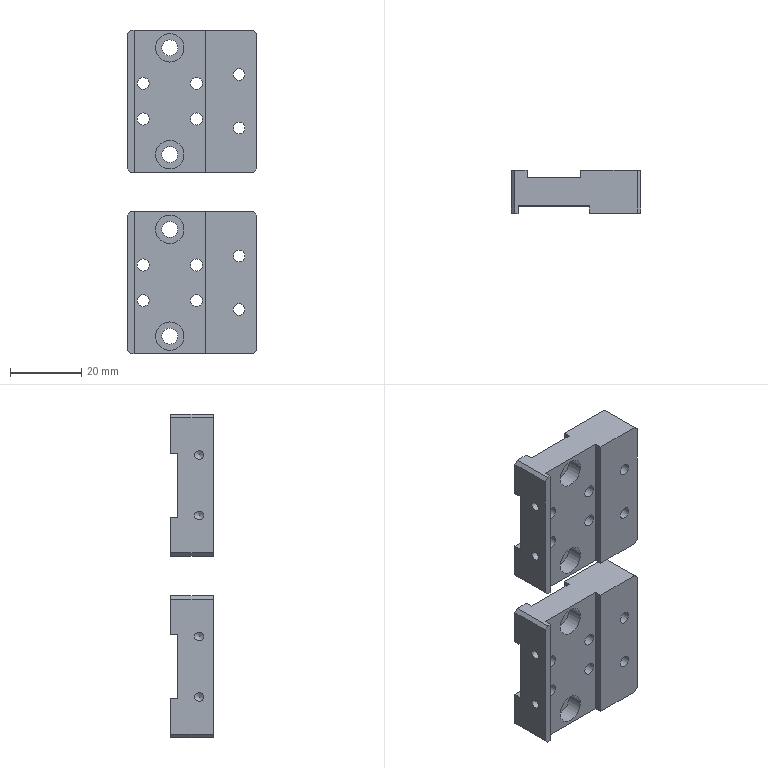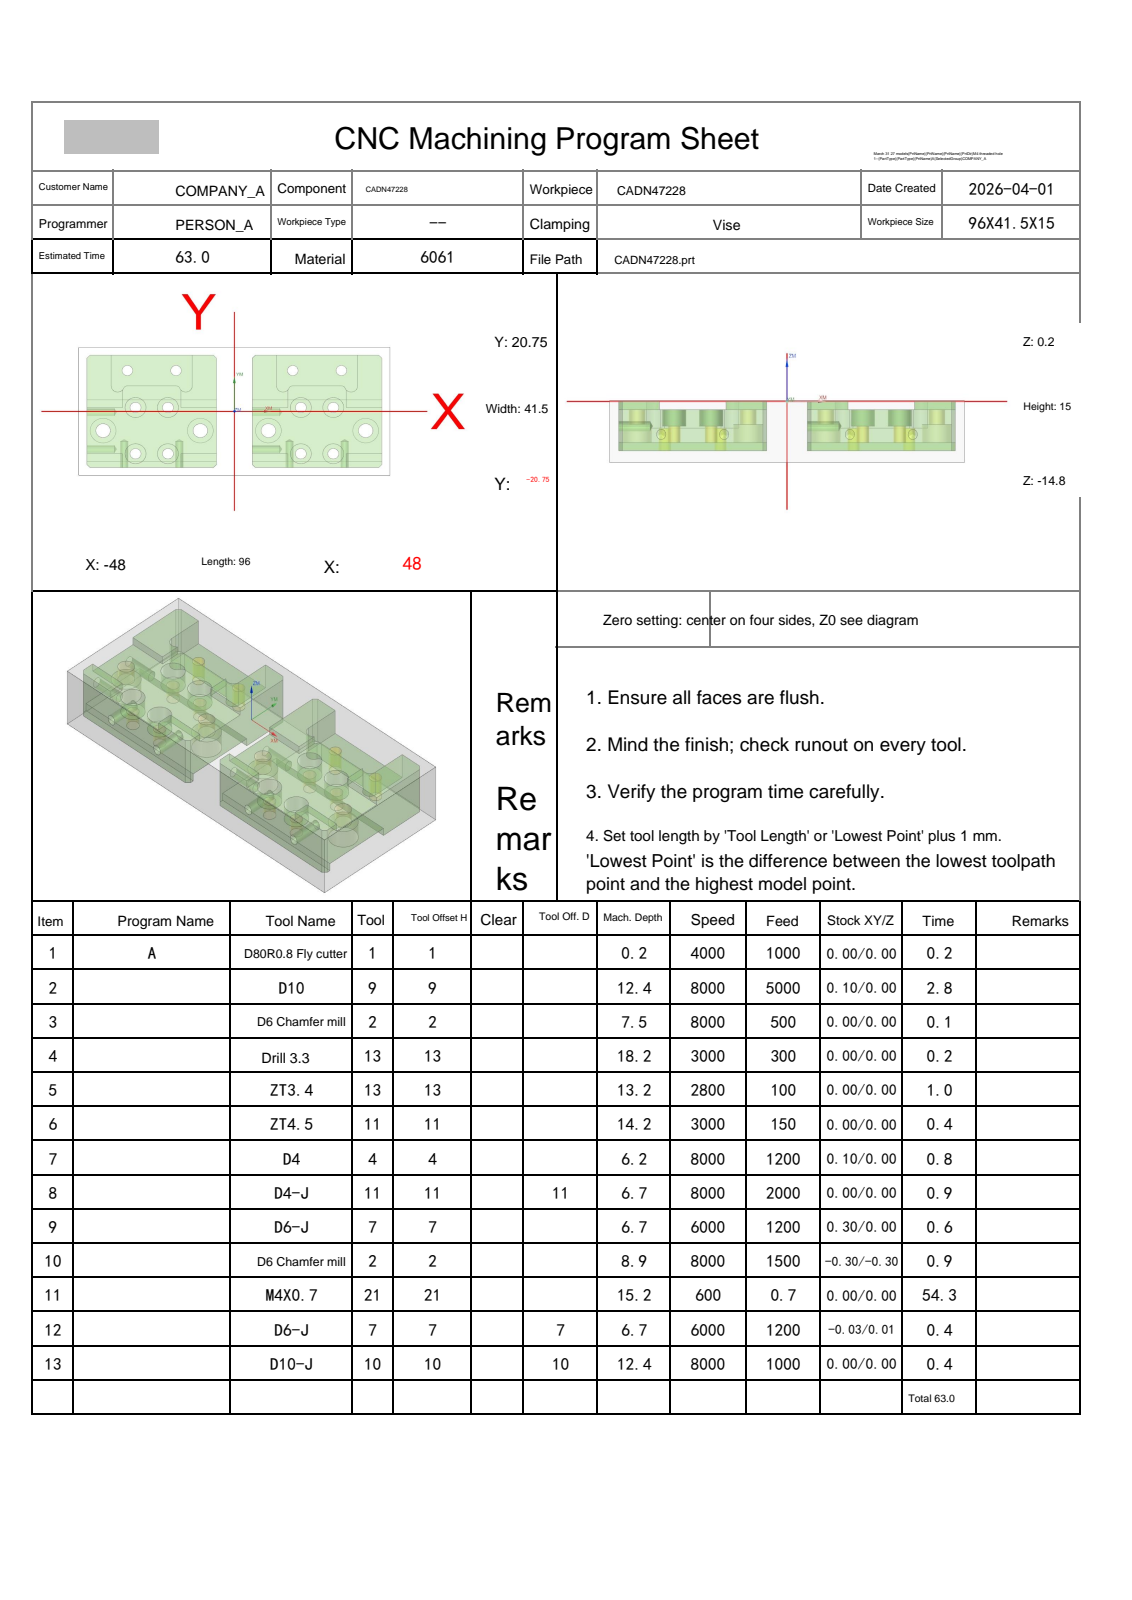NC program | NX | posted by the shop | part box 36.5 x 12 x 91 mm
Lines 1 to 1839 of 5439, first 1534 of 1837 lines:
%
O0001
(Machine time: 113.94 MIN)
(===Total Tool:9===)
(T1=D80R0.8 Fly cutter D=80.  R=0.8  D-  H01 Z=-0.   )
(T9=D10     D=10.  R=0.   D-  H09 Z=-12.2 )
(T2=D6 Chamfer mill   D=6.   R=0.   D-  H02 Z=-8.7  )
(T13=Drill 3.3  D=3.3  DR_a=118 D-  H13 Z=-17.99)
(T11=ZT4.5  D=4.5  DR_a=118 D-  H11 Z=-14.  )
(T4=D4      D=4.   R=0.   D-  H04 Z=-6.   )
(T7=D6-J    D=6.   R=0.   D-  H07 Z=-6.5  )
(T21=M4X0.7 D=3.3  DR_a=180 D-  H21 Z=-15.  )
(T10=D10-J  D=10.  R=0.   D10 H10 Z=-12.2 )
G80 G90 G17 G49 G40
G91 G28 Z0
M01
N1 T01 M06
(D80R0.8 Fly cutter  D=80. R=0.8 H=01 ce=0.00 di=0.00)
G00 G90 G54 X90.5 Y0.0 M03 S4000
G43 H01 Z20.
M08
Z2.
G01 Z0.0 F1000.
X85.5
X-85.5
X-90.5
Z2.
G00 Z20.
G91 G28 Z0.0
M05
M09
G91 G28 Z0.0
M01
N2 T09 M06
(D10  D=10. R=0. H=09 ce=0.10 di=0.00)
G00 G90 G54 X25.5 Y23.35 M03 S8000
G43 H09 Z20.
M08
Z.5
G01 X44.5 Z.449 F5000.
G02 X48.106 Y21.856 Z.438 I0.0 J-5.1
G01 X49.106 Y20.856 Z.435
G02 X50.6 Y17.25 Z.424 I-3.606 J-3.606
G01 Y-17.25 Z.332
G02 X49.106 Y-20.856 Z.321 I-5.1 J0.0
G01 X48.106 Y-21.856 Z.317
G02 X44.5 Y-23.35 Z.307 I-3.606 J3.606
G01 X6.5 Z.205
G02 X2.894 Y-21.856 Z.194 I0.0 J5.1
G01 X1.894 Y-20.856 Z.19
G02 X.4 Y-17.25 Z.18 I3.606 J3.606
G01 Y17.25 Z.088
G02 X1.894 Y20.856 Z.077 I5.1 J0.0
G01 X2.894 Y21.856 Z.073
G02 X6.5 Y23.35 Z.062 I3.606 J-3.606
G01 X44.5 Z-.039
G02 X48.106 Y21.856 Z-.05 I0.0 J-5.1
G01 X49.106 Y20.856 Z-.054
G02 X50.6 Y17.25 Z-.064 I-3.606 J-3.606
G01 Y-17.25 Z-.157
G02 X49.106 Y-20.856 Z-.167 I-5.1 J0.0
G01 X48.106 Y-21.856 Z-.171
G02 X44.5 Y-23.35 Z-.182 I-3.606 J3.606
G01 X6.5 Z-.283
G02 X2.894 Y-21.856 Z-.294 I0.0 J5.1
G01 X1.894 Y-20.856 Z-.298
G02 X.4 Y-17.25 Z-.309 I3.606 J3.606
G01 Y17.25 Z-.401
G02 X1.894 Y20.856 Z-.412 I5.1 J0.0
G01 X2.894 Y21.856 Z-.415
G02 X6.5 Y23.35 Z-.426 I3.606 J-3.606
G01 X44.5 Z-.528
G02 X48.106 Y21.856 Z-.538 I0.0 J-5.1
G01 X49.106 Y20.856 Z-.542
G02 X50.6 Y17.25 Z-.553 I-3.606 J-3.606
G01 Y-17.25 Z-.645
G02 X49.106 Y-20.856 Z-.656 I-5.1 J0.0
G01 X48.106 Y-21.856 Z-.66
G02 X44.5 Y-23.35 Z-.67 I-3.606 J3.606
G01 X6.5 Z-.772
G02 X2.894 Y-21.856 Z-.783 I0.0 J5.1
G01 X1.894 Y-20.856 Z-.786
G02 X.4 Y-17.25 Z-.797 I3.606 J3.606
G01 Y17.25 Z-.889
G02 X1.894 Y20.856 Z-.9 I5.1 J0.0
G01 X2.894 Y21.856 Z-.904
G02 X6.5 Y23.35 Z-.915 I3.606 J-3.606
G01 X44.5 Z-1.016
G02 X48.106 Y21.856 Z-1.027 I0.0 J-5.1
G01 X49.106 Y20.856 Z-1.031
G02 X50.6 Y17.25 Z-1.041 I-3.606 J-3.606
G01 Y-17.25 Z-1.134
G02 X49.106 Y-20.856 Z-1.144 I-5.1 J0.0
G01 X48.106 Y-21.856 Z-1.148
G02 X44.5 Y-23.35 Z-1.159 I-3.606 J3.606
G01 X6.5 Z-1.26
G02 X2.894 Y-21.856 Z-1.271 I0.0 J5.1
G01 X1.894 Y-20.856 Z-1.275
G02 X.4 Y-17.25 Z-1.286 I3.606 J3.606
G01 Y17.25 Z-1.378
G02 X1.894 Y20.856 Z-1.389 I5.1 J0.0
G01 X2.894 Y21.856 Z-1.392
G02 X6.5 Y23.35 Z-1.403 I3.606 J-3.606
G01 X44.5 Z-1.505
G02 X48.106 Y21.856 Z-1.515 I0.0 J-5.1
G01 X49.106 Y20.856 Z-1.519
G02 X50.6 Y17.25 Z-1.53 I-3.606 J-3.606
G01 Y-17.25 Z-1.622
G02 X49.106 Y-20.856 Z-1.633 I-5.1 J0.0
G01 X48.106 Y-21.856 Z-1.637
G02 X44.5 Y-23.35 Z-1.647 I-3.606 J3.606
G01 X6.5 Z-1.749
G02 X2.894 Y-21.856 Z-1.76 I0.0 J5.1
G01 X1.894 Y-20.856 Z-1.763
G02 X.4 Y-17.25 Z-1.774 I3.606 J3.606
G01 Y17.25 Z-1.866
G02 X1.894 Y20.856 Z-1.877 I5.1 J0.0
G01 X2.894 Y21.856 Z-1.881
G02 X6.5 Y23.35 Z-1.892 I3.606 J-3.606
G01 X44.5 Z-1.993
G02 X48.106 Y21.856 Z-2.004 I0.0 J-5.1
G01 X49.106 Y20.856 Z-2.008
G02 X50.6 Y17.25 Z-2.018 I-3.606 J-3.606
G01 Y-17.25 Z-2.111
G02 X49.106 Y-20.856 Z-2.121 I-5.1 J0.0
G01 X48.106 Y-21.856 Z-2.125
G02 X44.5 Y-23.35 Z-2.136 I-3.606 J3.606
G01 X6.5 Z-2.237
G02 X2.894 Y-21.856 Z-2.248 I0.0 J5.1
G01 X1.894 Y-20.856 Z-2.252
G02 X.4 Y-17.25 Z-2.263 I3.606 J3.606
G01 Y17.25 Z-2.355
G02 X1.894 Y20.856 Z-2.365 I5.1 J0.0
G01 X2.894 Y21.856 Z-2.369
G02 X6.5 Y23.35 Z-2.38 I3.606 J-3.606
G01 X44.5 Z-2.482
G02 X48.106 Y21.856 Z-2.492 I0.0 J-5.1
G01 X49.106 Y20.856 Z-2.496
G02 X50.6 Y17.25 Z-2.507 I-3.606 J-3.606
G01 Y-17.25 Z-2.599
G02 X49.106 Y-20.856 Z-2.61 I-5.1 J0.0
G01 X48.106 Y-21.856 Z-2.613
G02 X44.5 Y-23.35 Z-2.624 I-3.606 J3.606
G01 X6.5 Z-2.726
G02 X2.894 Y-21.856 Z-2.737 I0.0 J5.1
G01 X1.894 Y-20.856 Z-2.74
G02 X.4 Y-17.25 Z-2.751 I3.606 J3.606
G01 Y17.25 Z-2.843
G02 X1.894 Y20.856 Z-2.854 I5.1 J0.0
G01 X2.894 Y21.856 Z-2.858
G02 X6.5 Y23.35 Z-2.868 I3.606 J-3.606
G01 X44.5 Z-2.97
G02 X48.106 Y21.856 Z-2.981 I0.0 J-5.1
G01 X49.106 Y20.856 Z-2.985
G02 X50.6 Y17.25 Z-2.995 I-3.606 J-3.606
G01 Y-17.25 Z-3.087
G02 X49.106 Y-20.856 Z-3.098 I-5.1 J0.0
G01 X48.106 Y-21.856 Z-3.102
G02 X44.5 Y-23.35 Z-3.113 I-3.606 J3.606
G01 X6.5 Z-3.214
G02 X2.894 Y-21.856 Z-3.225 I0.0 J5.1
G01 X1.894 Y-20.856 Z-3.229
G02 X.4 Y-17.25 Z-3.239 I3.606 J3.606
G01 Y17.25 Z-3.332
G02 X1.894 Y20.856 Z-3.342 I5.1 J0.0
G01 X2.894 Y21.856 Z-3.346
G02 X6.5 Y23.35 Z-3.357 I3.606 J-3.606
G01 X44.5 Z-3.458
G02 X48.106 Y21.856 Z-3.469 I0.0 J-5.1
G01 X49.106 Y20.856 Z-3.473
G02 X50.6 Y17.25 Z-3.484 I-3.606 J-3.606
G01 Y-17.25 Z-3.576
G02 X49.106 Y-20.856 Z-3.587 I-5.1 J0.0
G01 X48.106 Y-21.856 Z-3.59
G02 X44.5 Y-23.35 Z-3.601 I-3.606 J3.606
G01 X6.5 Z-3.703
G02 X2.894 Y-21.856 Z-3.713 I0.0 J5.1
G01 X1.894 Y-20.856 Z-3.717
G02 X.4 Y-17.25 Z-3.728 I3.606 J3.606
G01 Y17.25 Z-3.82
G02 X1.894 Y20.856 Z-3.831 I5.1 J0.0
G01 X2.894 Y21.856 Z-3.835
G02 X6.5 Y23.35 Z-3.845 I3.606 J-3.606
G01 X44.5 Z-3.947
G02 X48.106 Y21.856 Z-3.958 I0.0 J-5.1
G01 X49.106 Y20.856 Z-3.961
G02 X50.6 Y17.25 Z-3.972 I-3.606 J-3.606
G01 Y-17.25 Z-4.064
G02 X49.106 Y-20.856 Z-4.075 I-5.1 J0.0
G01 X48.106 Y-21.856 Z-4.079
G02 X44.5 Y-23.35 Z-4.09 I-3.606 J3.606
G01 X6.5 Z-4.191
G02 X2.894 Y-21.856 Z-4.202 I0.0 J5.1
G01 X1.894 Y-20.856 Z-4.206
G02 X.4 Y-17.25 Z-4.216 I3.606 J3.606
G01 Y17.25 Z-4.309
G02 X1.894 Y20.856 Z-4.319 I5.1 J0.0
G01 X2.894 Y21.856 Z-4.323
G02 X6.5 Y23.35 Z-4.334 I3.606 J-3.606
G01 X44.5 Z-4.435
G02 X48.106 Y21.856 Z-4.446 I0.0 J-5.1
G01 X49.106 Y20.856 Z-4.45
G02 X50.6 Y17.25 Z-4.461 I-3.606 J-3.606
G01 Y-17.25 Z-4.553
G02 X49.106 Y-20.856 Z-4.564 I-5.1 J0.0
G01 X48.106 Y-21.856 Z-4.567
G02 X44.5 Y-23.35 Z-4.578 I-3.606 J3.606
G01 X6.5 Z-4.68
G02 X2.894 Y-21.856 Z-4.69 I0.0 J5.1
G01 X1.894 Y-20.856 Z-4.694
G02 X.4 Y-17.25 Z-4.705 I3.606 J3.606
G01 Y17.25 Z-4.797
G02 X1.894 Y20.856 Z-4.808 I5.1 J0.0
G01 X2.894 Y21.856 Z-4.812
G02 X6.5 Y23.35 Z-4.822 I3.606 J-3.606
G01 X44.5 Z-4.924
G02 X48.106 Y21.856 Z-4.935 I0.0 J-5.1
G01 X49.106 Y20.856 Z-4.938
G02 X50.6 Y17.25 Z-4.949 I-3.606 J-3.606
G01 Y-17.25 Z-5.041
G02 X49.106 Y-20.856 Z-5.052 I-5.1 J0.0
G01 X48.106 Y-21.856 Z-5.056
G02 X44.5 Y-23.35 Z-5.067 I-3.606 J3.606
G01 X6.5 Z-5.168
G02 X2.894 Y-21.856 Z-5.179 I0.0 J5.1
G01 X1.894 Y-20.856 Z-5.183
G02 X.4 Y-17.25 Z-5.193 I3.606 J3.606
G01 Y17.25 Z-5.286
G02 X1.894 Y20.856 Z-5.296 I5.1 J0.0
G01 X2.894 Y21.856 Z-5.3
G02 X6.5 Y23.35 Z-5.311 I3.606 J-3.606
G01 X44.5 Z-5.412
G02 X48.106 Y21.856 Z-5.423 I0.0 J-5.1
G01 X49.106 Y20.856 Z-5.427
G02 X50.6 Y17.25 Z-5.438 I-3.606 J-3.606
G01 Y-17.25 Z-5.53
G02 X49.106 Y-20.856 Z-5.54 I-5.1 J0.0
G01 X48.106 Y-21.856 Z-5.544
G02 X44.5 Y-23.35 Z-5.555 I-3.606 J3.606
G01 X6.5 Z-5.657
G02 X2.894 Y-21.856 Z-5.667 I0.0 J5.1
G01 X1.894 Y-20.856 Z-5.671
G02 X.4 Y-17.25 Z-5.682 I3.606 J3.606
G01 Y17.25 Z-5.774
G02 X1.894 Y20.856 Z-5.785 I5.1 J0.0
G01 X2.894 Y21.856 Z-5.788
G02 X6.5 Y23.35 Z-5.799 I3.606 J-3.606
G01 X44.5 Z-5.901
G02 X48.106 Y21.856 Z-5.912 I0.0 J-5.1
G01 X49.106 Y20.856 Z-5.915
G02 X50.6 Y17.25 Z-5.926 I-3.606 J-3.606
G01 Y-17.25 Z-6.018
G02 X49.106 Y-20.856 Z-6.029 I-5.1 J0.0
G01 X48.106 Y-21.856 Z-6.033
G02 X44.5 Y-23.35 Z-6.043 I-3.606 J3.606
G01 X6.5 Z-6.145
G02 X2.894 Y-21.856 Z-6.156 I0.0 J5.1
G01 X1.894 Y-20.856 Z-6.16
G02 X.4 Y-17.25 Z-6.17 I3.606 J3.606
G01 Y17.25 Z-6.262
G02 X1.894 Y20.856 Z-6.273 I5.1 J0.0
G01 X2.894 Y21.856 Z-6.277
G02 X6.5 Y23.35 Z-6.288 I3.606 J-3.606
G01 X44.5 Z-6.389
G02 X48.106 Y21.856 Z-6.4 I0.0 J-5.1
G01 X49.106 Y20.856 Z-6.404
G02 X50.6 Y17.25 Z-6.414 I-3.606 J-3.606
G01 Y-17.25 Z-6.507
G02 X49.106 Y-20.856 Z-6.517 I-5.1 J0.0
G01 X48.106 Y-21.856 Z-6.521
G02 X44.5 Y-23.35 Z-6.532 I-3.606 J3.606
G01 X6.5 Z-6.633
G02 X2.894 Y-21.856 Z-6.644 I0.0 J5.1
G01 X1.894 Y-20.856 Z-6.648
G02 X.4 Y-17.25 Z-6.659 I3.606 J3.606
G01 Y17.25 Z-6.751
G02 X1.894 Y20.856 Z-6.762 I5.1 J0.0
G01 X2.894 Y21.856 Z-6.765
G02 X6.5 Y23.35 Z-6.776 I3.606 J-3.606
G01 X44.5 Z-6.878
G02 X48.106 Y21.856 Z-6.888 I0.0 J-5.1
G01 X49.106 Y20.856 Z-6.892
G02 X50.6 Y17.25 Z-6.903 I-3.606 J-3.606
G01 Y-17.25 Z-6.995
G02 X49.106 Y-20.856 Z-7.006 I-5.1 J0.0
G01 X48.106 Y-21.856 Z-7.01
G02 X44.5 Y-23.35 Z-7.02 I-3.606 J3.606
G01 X6.5 Z-7.122
G02 X2.894 Y-21.856 Z-7.133 I0.0 J5.1
G01 X1.894 Y-20.856 Z-7.136
G02 X.4 Y-17.25 Z-7.147 I3.606 J3.606
G01 Y17.25 Z-7.239
G02 X1.894 Y20.856 Z-7.25 I5.1 J0.0
G01 X2.894 Y21.856 Z-7.254
G02 X6.5 Y23.35 Z-7.265 I3.606 J-3.606
G01 X44.5 Z-7.366
G02 X48.106 Y21.856 Z-7.377 I0.0 J-5.1
G01 X49.106 Y20.856 Z-7.381
G02 X50.6 Y17.25 Z-7.391 I-3.606 J-3.606
G01 Y-17.25 Z-7.484
G02 X49.106 Y-20.856 Z-7.494 I-5.1 J0.0
G01 X48.106 Y-21.856 Z-7.498
G02 X44.5 Y-23.35 Z-7.509 I-3.606 J3.606
G01 X6.5 Z-7.61
G02 X2.894 Y-21.856 Z-7.621 I0.0 J5.1
G01 X1.894 Y-20.856 Z-7.625
G02 X.4 Y-17.25 Z-7.636 I3.606 J3.606
G01 Y17.25 Z-7.728
G02 X1.894 Y20.856 Z-7.739 I5.1 J0.0
G01 X2.894 Y21.856 Z-7.742
G02 X6.5 Y23.35 Z-7.753 I3.606 J-3.606
G01 X44.5 Z-7.855
G02 X48.106 Y21.856 Z-7.865 I0.0 J-5.1
G01 X49.106 Y20.856 Z-7.869
G02 X50.6 Y17.25 Z-7.88 I-3.606 J-3.606
G01 Y-17.25 Z-7.972
G02 X49.106 Y-20.856 Z-7.983 I-5.1 J0.0
G01 X48.106 Y-21.856 Z-7.987
G02 X44.5 Y-23.35 Z-7.997 I-3.606 J3.606
G01 X6.5 Z-8.099
G02 X2.894 Y-21.856 Z-8.11 I0.0 J5.1
G01 X1.894 Y-20.856 Z-8.113
G02 X.4 Y-17.25 Z-8.124 I3.606 J3.606
G01 Y17.25 Z-8.216
G02 X1.894 Y20.856 Z-8.227 I5.1 J0.0
G01 X2.894 Y21.856 Z-8.231
G02 X6.5 Y23.35 Z-8.242 I3.606 J-3.606
G01 X44.5 Z-8.343
G02 X48.106 Y21.856 Z-8.354 I0.0 J-5.1
G01 X49.106 Y20.856 Z-8.358
G02 X50.6 Y17.25 Z-8.368 I-3.606 J-3.606
G01 Y-17.25 Z-8.461
G02 X49.106 Y-20.856 Z-8.471 I-5.1 J0.0
G01 X48.106 Y-21.856 Z-8.475
G02 X44.5 Y-23.35 Z-8.486 I-3.606 J3.606
G01 X6.5 Z-8.587
G02 X2.894 Y-21.856 Z-8.598 I0.0 J5.1
G01 X1.894 Y-20.856 Z-8.602
G02 X.4 Y-17.25 Z-8.613 I3.606 J3.606
G01 Y17.25 Z-8.705
G02 X1.894 Y20.856 Z-8.715 I5.1 J0.0
G01 X2.894 Y21.856 Z-8.719
G02 X6.5 Y23.35 Z-8.73 I3.606 J-3.606
G01 X44.5 Z-8.832
G02 X48.106 Y21.856 Z-8.842 I0.0 J-5.1
G01 X49.106 Y20.856 Z-8.846
G02 X50.6 Y17.25 Z-8.857 I-3.606 J-3.606
G01 Y-17.25 Z-8.949
G02 X49.106 Y-20.856 Z-8.96 I-5.1 J0.0
G01 X48.106 Y-21.856 Z-8.963
G02 X44.5 Y-23.35 Z-8.974 I-3.606 J3.606
G01 X6.5 Z-9.076
G02 X2.894 Y-21.856 Z-9.087 I0.0 J5.1
G01 X1.894 Y-20.856 Z-9.09
G02 X.4 Y-17.25 Z-9.101 I3.606 J3.606
G01 Y17.25 Z-9.193
G02 X1.894 Y20.856 Z-9.204 I5.1 J0.0
G01 X2.894 Y21.856 Z-9.208
G02 X6.5 Y23.35 Z-9.218 I3.606 J-3.606
G01 X44.5 Z-9.32
G02 X48.106 Y21.856 Z-9.331 I0.0 J-5.1
G01 X49.106 Y20.856 Z-9.335
G02 X50.6 Y17.25 Z-9.345 I-3.606 J-3.606
G01 Y-17.25 Z-9.437
G02 X49.106 Y-20.856 Z-9.448 I-5.1 J0.0
G01 X48.106 Y-21.856 Z-9.452
G02 X44.5 Y-23.35 Z-9.463 I-3.606 J3.606
G01 X6.5 Z-9.564
G02 X2.894 Y-21.856 Z-9.575 I0.0 J5.1
G01 X1.894 Y-20.856 Z-9.579
G02 X.4 Y-17.25 Z-9.589 I3.606 J3.606
G01 Y17.25 Z-9.682
G02 X1.894 Y20.856 Z-9.692 I5.1 J0.0
G01 X2.894 Y21.856 Z-9.696
G02 X6.5 Y23.35 Z-9.707 I3.606 J-3.606
G01 X44.5 Z-9.808
G02 X48.106 Y21.856 Z-9.819 I0.0 J-5.1
G01 X49.106 Y20.856 Z-9.823
G02 X50.6 Y17.25 Z-9.834 I-3.606 J-3.606
G01 Y-17.25 Z-9.926
G02 X49.106 Y-20.856 Z-9.937 I-5.1 J0.0
G01 X48.106 Y-21.856 Z-9.94
G02 X44.5 Y-23.35 Z-9.951 I-3.606 J3.606
G01 X6.5 Z-10.053
G02 X2.894 Y-21.856 Z-10.063 I0.0 J5.1
G01 X1.894 Y-20.856 Z-10.067
G02 X.4 Y-17.25 Z-10.078 I3.606 J3.606
G01 Y17.25 Z-10.17
G02 X1.894 Y20.856 Z-10.181 I5.1 J0.0
G01 X2.894 Y21.856 Z-10.185
G02 X6.5 Y23.35 Z-10.195 I3.606 J-3.606
G01 X44.5 Z-10.297
G02 X48.106 Y21.856 Z-10.308 I0.0 J-5.1
G01 X49.106 Y20.856 Z-10.311
G02 X50.6 Y17.25 Z-10.322 I-3.606 J-3.606
G01 Y-17.25 Z-10.414
G02 X49.106 Y-20.856 Z-10.425 I-5.1 J0.0
G01 X48.106 Y-21.856 Z-10.429
G02 X44.5 Y-23.35 Z-10.44 I-3.606 J3.606
G01 X6.5 Z-10.541
G02 X2.894 Y-21.856 Z-10.552 I0.0 J5.1
G01 X1.894 Y-20.856 Z-10.556
G02 X.4 Y-17.25 Z-10.566 I3.606 J3.606
G01 Y17.25 Z-10.659
G02 X1.894 Y20.856 Z-10.669 I5.1 J0.0
G01 X2.894 Y21.856 Z-10.673
G02 X6.5 Y23.35 Z-10.684 I3.606 J-3.606
G01 X44.5 Z-10.785
G02 X48.106 Y21.856 Z-10.796 I0.0 J-5.1
G01 X49.106 Y20.856 Z-10.8
G02 X50.6 Y17.25 Z-10.811 I-3.606 J-3.606
G01 Y-17.25 Z-10.903
G02 X49.106 Y-20.856 Z-10.914 I-5.1 J0.0
G01 X48.106 Y-21.856 Z-10.917
G02 X44.5 Y-23.35 Z-10.928 I-3.606 J3.606
G01 X6.5 Z-11.03
G02 X2.894 Y-21.856 Z-11.04 I0.0 J5.1
G01 X1.894 Y-20.856 Z-11.044
G02 X.4 Y-17.25 Z-11.055 I3.606 J3.606
G01 Y17.25 Z-11.147
G02 X1.894 Y20.856 Z-11.158 I5.1 J0.0
G01 X2.894 Y21.856 Z-11.162
G02 X6.5 Y23.35 Z-11.172 I3.606 J-3.606
G01 X44.5 Z-11.274
G02 X48.106 Y21.856 Z-11.285 I0.0 J-5.1
G01 X49.106 Y20.856 Z-11.288
G02 X50.6 Y17.25 Z-11.299 I-3.606 J-3.606
G01 Y-17.25 Z-11.391
G02 X49.106 Y-20.856 Z-11.402 I-5.1 J0.0
G01 X48.106 Y-21.856 Z-11.406
G02 X44.5 Y-23.35 Z-11.417 I-3.606 J3.606
G01 X6.5 Z-11.518
G02 X2.894 Y-21.856 Z-11.529 I0.0 J5.1
G01 X1.894 Y-20.856 Z-11.533
G02 X.4 Y-17.25 Z-11.543 I3.606 J3.606
G01 Y17.25 Z-11.636
G02 X1.894 Y20.856 Z-11.646 I5.1 J0.0
G01 X2.894 Y21.856 Z-11.65
G02 X6.5 Y23.35 Z-11.661 I3.606 J-3.606
G01 X44.5 Z-11.762
G02 X48.106 Y21.856 Z-11.773 I0.0 J-5.1
G01 X49.106 Y20.856 Z-11.777
G02 X50.6 Y17.25 Z-11.788 I-3.606 J-3.606
G01 Y-17.25 Z-11.88
G02 X49.106 Y-20.856 Z-11.89 I-5.1 J0.0
G01 X48.106 Y-21.856 Z-11.894
G02 X44.5 Y-23.35 Z-11.905 I-3.606 J3.606
G01 X6.5 Z-12.007
G02 X2.894 Y-21.856 Z-12.017 I0.0 J5.1
G01 X1.894 Y-20.856 Z-12.021
G02 X.4 Y-17.25 Z-12.032 I3.606 J3.606
G01 Y17.25 Z-12.124
G02 X1.894 Y20.856 Z-12.135 I5.1 J0.0
G01 X2.894 Y21.856 Z-12.138
G02 X6.5 Y23.35 Z-12.149 I3.606 J-3.606
G01 X25.5 Z-12.2
X44.5
G02 X48.106 Y21.856 I0.0 J-5.1
G01 X49.106 Y20.856
G02 X50.6 Y17.25 I-3.606 J-3.606
G01 Y-17.25
G02 X49.106 Y-20.856 I-5.1 J0.0
G01 X48.106 Y-21.856
G02 X44.5 Y-23.35 I-3.606 J3.606
G01 X6.5
G02 X2.894 Y-21.856 I0.0 J5.1
G01 X1.894 Y-20.856
G02 X.4 Y-17.25 I3.606 J3.606
G01 Y17.25
G02 X1.894 Y20.856 I5.1 J0.0
G01 X2.894 Y21.856
G02 X6.5 Y23.35 I3.606 J-3.606
G01 X25.5
X26.
Z-11.2
G00 Z20.
X-25.5
Z.5
G01 X-6.5 Z.449
G02 X-2.894 Y21.856 Z.438 I0.0 J-5.1
G01 X-1.894 Y20.856 Z.435
G02 X-.409 Y17.547 Z.425 I-3.606 J-3.606
X-.4 Y17.25 Z.424 I-5.091 J-.297
G01 Y-17.25 Z.332
G02 X-1.894 Y-20.856 Z.321 I-5.1 J0.0
G01 X-2.894 Y-21.856 Z.317
G02 X-6.5 Y-23.35 Z.307 I-3.606 J3.606
G01 X-44.5 Z.205
G02 X-48.106 Y-21.856 Z.194 I0.0 J5.1
G01 X-49.106 Y-20.856 Z.19
G02 X-50.6 Y-17.25 Z.18 I3.606 J3.606
G01 Y17.25 Z.088
G02 X-49.106 Y20.856 Z.077 I5.1 J0.0
G01 X-48.106 Y21.856 Z.073
G02 X-44.5 Y23.35 Z.062 I3.606 J-3.606
G01 X-6.5 Z-.039
G02 X-2.894 Y21.856 Z-.05 I0.0 J-5.1
G01 X-1.894 Y20.856 Z-.054
G02 X-.409 Y17.547 Z-.064 I-3.606 J-3.606
X-.4 Y17.25 Z-.064 I-5.091 J-.297
G01 Y-17.25 Z-.157
G02 X-1.894 Y-20.856 Z-.167 I-5.1 J0.0
G01 X-2.894 Y-21.856 Z-.171
G02 X-6.5 Y-23.35 Z-.182 I-3.606 J3.606
G01 X-44.5 Z-.283
G02 X-48.106 Y-21.856 Z-.294 I0.0 J5.1
G01 X-49.106 Y-20.856 Z-.298
G02 X-50.6 Y-17.25 Z-.309 I3.606 J3.606
G01 Y17.25 Z-.401
G02 X-49.106 Y20.856 Z-.412 I5.1 J0.0
G01 X-48.106 Y21.856 Z-.415
G02 X-44.5 Y23.35 Z-.426 I3.606 J-3.606
G01 X-6.5 Z-.528
G02 X-2.894 Y21.856 Z-.538 I0.0 J-5.1
G01 X-1.894 Y20.856 Z-.542
G02 X-.409 Y17.547 Z-.552 I-3.606 J-3.606
X-.4 Y17.25 Z-.553 I-5.091 J-.297
G01 Y-17.25 Z-.645
G02 X-1.894 Y-20.856 Z-.656 I-5.1 J0.0
G01 X-2.894 Y-21.856 Z-.66
G02 X-6.5 Y-23.35 Z-.67 I-3.606 J3.606
G01 X-44.5 Z-.772
G02 X-48.106 Y-21.856 Z-.783 I0.0 J5.1
G01 X-49.106 Y-20.856 Z-.786
G02 X-50.6 Y-17.25 Z-.797 I3.606 J3.606
G01 Y17.25 Z-.889
G02 X-49.106 Y20.856 Z-.9 I5.1 J0.0
G01 X-48.106 Y21.856 Z-.904
G02 X-44.5 Y23.35 Z-.915 I3.606 J-3.606
G01 X-6.5 Z-1.016
G02 X-2.894 Y21.856 Z-1.027 I0.0 J-5.1
G01 X-1.894 Y20.856 Z-1.031
G02 X-.409 Y17.547 Z-1.041 I-3.606 J-3.606
X-.4 Y17.25 Z-1.041 I-5.091 J-.297
G01 Y-17.25 Z-1.134
G02 X-1.894 Y-20.856 Z-1.144 I-5.1 J0.0
G01 X-2.894 Y-21.856 Z-1.148
G02 X-6.5 Y-23.35 Z-1.159 I-3.606 J3.606
G01 X-44.5 Z-1.26
G02 X-48.106 Y-21.856 Z-1.271 I0.0 J5.1
G01 X-49.106 Y-20.856 Z-1.275
G02 X-50.6 Y-17.25 Z-1.286 I3.606 J3.606
G01 Y17.25 Z-1.378
G02 X-49.106 Y20.856 Z-1.389 I5.1 J0.0
G01 X-48.106 Y21.856 Z-1.392
G02 X-44.5 Y23.35 Z-1.403 I3.606 J-3.606
G01 X-6.5 Z-1.505
G02 X-2.894 Y21.856 Z-1.515 I0.0 J-5.1
G01 X-1.894 Y20.856 Z-1.519
G02 X-.409 Y17.547 Z-1.529 I-3.606 J-3.606
X-.4 Y17.25 Z-1.53 I-5.091 J-.297
G01 Y-17.25 Z-1.622
G02 X-1.894 Y-20.856 Z-1.633 I-5.1 J0.0
G01 X-2.894 Y-21.856 Z-1.637
G02 X-6.5 Y-23.35 Z-1.647 I-3.606 J3.606
G01 X-44.5 Z-1.749
G02 X-48.106 Y-21.856 Z-1.76 I0.0 J5.1
G01 X-49.106 Y-20.856 Z-1.763
G02 X-50.6 Y-17.25 Z-1.774 I3.606 J3.606
G01 Y17.25 Z-1.866
G02 X-49.106 Y20.856 Z-1.877 I5.1 J0.0
G01 X-48.106 Y21.856 Z-1.881
G02 X-44.5 Y23.35 Z-1.892 I3.606 J-3.606
G01 X-6.5 Z-1.993
G02 X-2.894 Y21.856 Z-2.004 I0.0 J-5.1
G01 X-1.894 Y20.856 Z-2.008
G02 X-.409 Y17.547 Z-2.018 I-3.606 J-3.606
X-.4 Y17.25 Z-2.018 I-5.091 J-.297
G01 Y-17.25 Z-2.111
G02 X-1.894 Y-20.856 Z-2.121 I-5.1 J0.0
G01 X-2.894 Y-21.856 Z-2.125
G02 X-6.5 Y-23.35 Z-2.136 I-3.606 J3.606
G01 X-44.5 Z-2.237
G02 X-48.106 Y-21.856 Z-2.248 I0.0 J5.1
G01 X-49.106 Y-20.856 Z-2.252
G02 X-50.6 Y-17.25 Z-2.263 I3.606 J3.606
G01 Y17.25 Z-2.355
G02 X-49.106 Y20.856 Z-2.365 I5.1 J0.0
G01 X-48.106 Y21.856 Z-2.369
G02 X-44.5 Y23.35 Z-2.38 I3.606 J-3.606
G01 X-6.5 Z-2.482
G02 X-2.894 Y21.856 Z-2.492 I0.0 J-5.1
G01 X-1.894 Y20.856 Z-2.496
G02 X-.409 Y17.547 Z-2.506 I-3.606 J-3.606
X-.4 Y17.25 Z-2.507 I-5.091 J-.297
G01 Y-17.25 Z-2.599
G02 X-1.894 Y-20.856 Z-2.61 I-5.1 J0.0
G01 X-2.894 Y-21.856 Z-2.613
G02 X-6.5 Y-23.35 Z-2.624 I-3.606 J3.606
G01 X-44.5 Z-2.726
G02 X-48.106 Y-21.856 Z-2.737 I0.0 J5.1
G01 X-49.106 Y-20.856 Z-2.74
G02 X-50.6 Y-17.25 Z-2.751 I3.606 J3.606
G01 Y17.25 Z-2.843
G02 X-49.106 Y20.856 Z-2.854 I5.1 J0.0
G01 X-48.106 Y21.856 Z-2.858
G02 X-44.5 Y23.35 Z-2.868 I3.606 J-3.606
G01 X-6.5 Z-2.97
G02 X-2.894 Y21.856 Z-2.981 I0.0 J-5.1
G01 X-1.894 Y20.856 Z-2.985
G02 X-.409 Y17.547 Z-2.994 I-3.606 J-3.606
X-.4 Y17.25 Z-2.995 I-5.091 J-.297
G01 Y-17.25 Z-3.087
G02 X-1.894 Y-20.856 Z-3.098 I-5.1 J0.0
G01 X-2.894 Y-21.856 Z-3.102
G02 X-6.5 Y-23.35 Z-3.113 I-3.606 J3.606
G01 X-44.5 Z-3.214
G02 X-48.106 Y-21.856 Z-3.225 I0.0 J5.1
G01 X-49.106 Y-20.856 Z-3.229
G02 X-50.6 Y-17.25 Z-3.239 I3.606 J3.606
G01 Y17.25 Z-3.332
G02 X-49.106 Y20.856 Z-3.342 I5.1 J0.0
G01 X-48.106 Y21.856 Z-3.346
G02 X-44.5 Y23.35 Z-3.357 I3.606 J-3.606
G01 X-6.5 Z-3.458
G02 X-2.894 Y21.856 Z-3.469 I0.0 J-5.1
G01 X-1.894 Y20.856 Z-3.473
G02 X-.409 Y17.547 Z-3.483 I-3.606 J-3.606
X-.4 Y17.25 Z-3.484 I-5.091 J-.297
G01 Y-17.25 Z-3.576
G02 X-1.894 Y-20.856 Z-3.587 I-5.1 J0.0
G01 X-2.894 Y-21.856 Z-3.59
G02 X-6.5 Y-23.35 Z-3.601 I-3.606 J3.606
G01 X-44.5 Z-3.703
G02 X-48.106 Y-21.856 Z-3.713 I0.0 J5.1
G01 X-49.106 Y-20.856 Z-3.717
G02 X-50.6 Y-17.25 Z-3.728 I3.606 J3.606
G01 Y17.25 Z-3.82
G02 X-49.106 Y20.856 Z-3.831 I5.1 J0.0
G01 X-48.106 Y21.856 Z-3.835
G02 X-44.5 Y23.35 Z-3.845 I3.606 J-3.606
G01 X-6.5 Z-3.947
G02 X-2.894 Y21.856 Z-3.958 I0.0 J-5.1
G01 X-1.894 Y20.856 Z-3.961
G02 X-.409 Y17.547 Z-3.971 I-3.606 J-3.606
X-.4 Y17.25 Z-3.972 I-5.091 J-.297
G01 Y-17.25 Z-4.064
G02 X-1.894 Y-20.856 Z-4.075 I-5.1 J0.0
G01 X-2.894 Y-21.856 Z-4.079
G02 X-6.5 Y-23.35 Z-4.09 I-3.606 J3.606
G01 X-44.5 Z-4.191
G02 X-48.106 Y-21.856 Z-4.202 I0.0 J5.1
G01 X-49.106 Y-20.856 Z-4.206
G02 X-50.6 Y-17.25 Z-4.216 I3.606 J3.606
G01 Y17.25 Z-4.309
G02 X-49.106 Y20.856 Z-4.319 I5.1 J0.0
G01 X-48.106 Y21.856 Z-4.323
G02 X-44.5 Y23.35 Z-4.334 I3.606 J-3.606
G01 X-6.5 Z-4.435
G02 X-2.894 Y21.856 Z-4.446 I0.0 J-5.1
G01 X-1.894 Y20.856 Z-4.45
G02 X-.409 Y17.547 Z-4.46 I-3.606 J-3.606
X-.4 Y17.25 Z-4.461 I-5.091 J-.297
G01 Y-17.25 Z-4.553
G02 X-1.894 Y-20.856 Z-4.564 I-5.1 J0.0
G01 X-2.894 Y-21.856 Z-4.567
G02 X-6.5 Y-23.35 Z-4.578 I-3.606 J3.606
G01 X-44.5 Z-4.68
G02 X-48.106 Y-21.856 Z-4.69 I0.0 J5.1
G01 X-49.106 Y-20.856 Z-4.694
G02 X-50.6 Y-17.25 Z-4.705 I3.606 J3.606
G01 Y17.25 Z-4.797
G02 X-49.106 Y20.856 Z-4.808 I5.1 J0.0
G01 X-48.106 Y21.856 Z-4.812
G02 X-44.5 Y23.35 Z-4.822 I3.606 J-3.606
G01 X-6.5 Z-4.924
G02 X-2.894 Y21.856 Z-4.935 I0.0 J-5.1
G01 X-1.894 Y20.856 Z-4.938
G02 X-.409 Y17.547 Z-4.948 I-3.606 J-3.606
X-.4 Y17.25 Z-4.949 I-5.091 J-.297
G01 Y-17.25 Z-5.041
G02 X-1.894 Y-20.856 Z-5.052 I-5.1 J0.0
G01 X-2.894 Y-21.856 Z-5.056
G02 X-6.5 Y-23.35 Z-5.067 I-3.606 J3.606
G01 X-44.5 Z-5.168
G02 X-48.106 Y-21.856 Z-5.179 I0.0 J5.1
G01 X-49.106 Y-20.856 Z-5.183
G02 X-50.6 Y-17.25 Z-5.193 I3.606 J3.606
G01 Y17.25 Z-5.286
G02 X-49.106 Y20.856 Z-5.296 I5.1 J0.0
G01 X-48.106 Y21.856 Z-5.3
G02 X-44.5 Y23.35 Z-5.311 I3.606 J-3.606
G01 X-6.5 Z-5.412
G02 X-2.894 Y21.856 Z-5.423 I0.0 J-5.1
G01 X-1.894 Y20.856 Z-5.427
G02 X-.409 Y17.547 Z-5.437 I-3.606 J-3.606
X-.4 Y17.25 Z-5.438 I-5.091 J-.297
G01 Y-17.25 Z-5.53
G02 X-1.894 Y-20.856 Z-5.54 I-5.1 J0.0
G01 X-2.894 Y-21.856 Z-5.544
G02 X-6.5 Y-23.35 Z-5.555 I-3.606 J3.606
G01 X-44.5 Z-5.657
G02 X-48.106 Y-21.856 Z-5.667 I0.0 J5.1
G01 X-49.106 Y-20.856 Z-5.671
G02 X-50.6 Y-17.25 Z-5.682 I3.606 J3.606
G01 Y17.25 Z-5.774
G02 X-49.106 Y20.856 Z-5.785 I5.1 J0.0
G01 X-48.106 Y21.856 Z-5.788
G02 X-44.5 Y23.35 Z-5.799 I3.606 J-3.606
G01 X-6.5 Z-5.901
G02 X-2.894 Y21.856 Z-5.912 I0.0 J-5.1
G01 X-1.894 Y20.856 Z-5.915
G02 X-.409 Y17.547 Z-5.925 I-3.606 J-3.606
X-.4 Y17.25 Z-5.926 I-5.091 J-.297
G01 Y-17.25 Z-6.018
G02 X-1.894 Y-20.856 Z-6.029 I-5.1 J0.0
G01 X-2.894 Y-21.856 Z-6.033
G02 X-6.5 Y-23.35 Z-6.043 I-3.606 J3.606
G01 X-44.5 Z-6.145
G02 X-48.106 Y-21.856 Z-6.156 I0.0 J5.1
G01 X-49.106 Y-20.856 Z-6.16
G02 X-50.6 Y-17.25 Z-6.17 I3.606 J3.606
G01 Y17.25 Z-6.262
G02 X-49.106 Y20.856 Z-6.273 I5.1 J0.0
G01 X-48.106 Y21.856 Z-6.277
G02 X-44.5 Y23.35 Z-6.288 I3.606 J-3.606
G01 X-6.5 Z-6.389
G02 X-2.894 Y21.856 Z-6.4 I0.0 J-5.1
G01 X-1.894 Y20.856 Z-6.404
G02 X-.409 Y17.547 Z-6.414 I-3.606 J-3.606
X-.4 Y17.25 Z-6.414 I-5.091 J-.297
G01 Y-17.25 Z-6.507
G02 X-1.894 Y-20.856 Z-6.517 I-5.1 J0.0
G01 X-2.894 Y-21.856 Z-6.521
G02 X-6.5 Y-23.35 Z-6.532 I-3.606 J3.606
G01 X-44.5 Z-6.633
G02 X-48.106 Y-21.856 Z-6.644 I0.0 J5.1
G01 X-49.106 Y-20.856 Z-6.648
G02 X-50.6 Y-17.25 Z-6.659 I3.606 J3.606
G01 Y17.25 Z-6.751
G02 X-49.106 Y20.856 Z-6.762 I5.1 J0.0
G01 X-48.106 Y21.856 Z-6.765
G02 X-44.5 Y23.35 Z-6.776 I3.606 J-3.606
G01 X-6.5 Z-6.878
G02 X-2.894 Y21.856 Z-6.888 I0.0 J-5.1
G01 X-1.894 Y20.856 Z-6.892
G02 X-.409 Y17.547 Z-6.902 I-3.606 J-3.606
X-.4 Y17.25 Z-6.903 I-5.091 J-.297
G01 Y-17.25 Z-6.995
G02 X-1.894 Y-20.856 Z-7.006 I-5.1 J0.0
G01 X-2.894 Y-21.856 Z-7.01
G02 X-6.5 Y-23.35 Z-7.02 I-3.606 J3.606
G01 X-44.5 Z-7.122
G02 X-48.106 Y-21.856 Z-7.133 I0.0 J5.1
G01 X-49.106 Y-20.856 Z-7.136
G02 X-50.6 Y-17.25 Z-7.147 I3.606 J3.606
G01 Y17.25 Z-7.239
G02 X-49.106 Y20.856 Z-7.25 I5.1 J0.0
G01 X-48.106 Y21.856 Z-7.254
G02 X-44.5 Y23.35 Z-7.265 I3.606 J-3.606
G01 X-6.5 Z-7.366
G02 X-2.894 Y21.856 Z-7.377 I0.0 J-5.1
G01 X-1.894 Y20.856 Z-7.381
G02 X-.409 Y17.547 Z-7.391 I-3.606 J-3.606
X-.4 Y17.25 Z-7.391 I-5.091 J-.297
G01 Y-17.25 Z-7.484
G02 X-1.894 Y-20.856 Z-7.494 I-5.1 J0.0
G01 X-2.894 Y-21.856 Z-7.498
G02 X-6.5 Y-23.35 Z-7.509 I-3.606 J3.606
G01 X-44.5 Z-7.61
G02 X-48.106 Y-21.856 Z-7.621 I0.0 J5.1
G01 X-49.106 Y-20.856 Z-7.625
G02 X-50.6 Y-17.25 Z-7.636 I3.606 J3.606
G01 Y17.25 Z-7.728
G02 X-49.106 Y20.856 Z-7.739 I5.1 J0.0
G01 X-48.106 Y21.856 Z-7.742
G02 X-44.5 Y23.35 Z-7.753 I3.606 J-3.606
G01 X-6.5 Z-7.855
G02 X-2.894 Y21.856 Z-7.865 I0.0 J-5.1
G01 X-1.894 Y20.856 Z-7.869
G02 X-.409 Y17.547 Z-7.879 I-3.606 J-3.606
X-.4 Y17.25 Z-7.88 I-5.091 J-.297
G01 Y-17.25 Z-7.972
G02 X-1.894 Y-20.856 Z-7.983 I-5.1 J0.0
G01 X-2.894 Y-21.856 Z-7.987
G02 X-6.5 Y-23.35 Z-7.997 I-3.606 J3.606
G01 X-44.5 Z-8.099
G02 X-48.106 Y-21.856 Z-8.11 I0.0 J5.1
G01 X-49.106 Y-20.856 Z-8.113
G02 X-50.6 Y-17.25 Z-8.124 I3.606 J3.606
G01 Y17.25 Z-8.216
G02 X-49.106 Y20.856 Z-8.227 I5.1 J0.0
G01 X-48.106 Y21.856 Z-8.231
G02 X-44.5 Y23.35 Z-8.242 I3.606 J-3.606
G01 X-6.5 Z-8.343
G02 X-2.894 Y21.856 Z-8.354 I0.0 J-5.1
G01 X-1.894 Y20.856 Z-8.358
G02 X-.409 Y17.547 Z-8.368 I-3.606 J-3.606
X-.4 Y17.25 Z-8.368 I-5.091 J-.297
G01 Y-17.25 Z-8.461
G02 X-1.894 Y-20.856 Z-8.471 I-5.1 J0.0
G01 X-2.894 Y-21.856 Z-8.475
G02 X-6.5 Y-23.35 Z-8.486 I-3.606 J3.606
G01 X-44.5 Z-8.587
G02 X-48.106 Y-21.856 Z-8.598 I0.0 J5.1
G01 X-49.106 Y-20.856 Z-8.602
G02 X-50.6 Y-17.25 Z-8.613 I3.606 J3.606
G01 Y17.25 Z-8.705
G02 X-49.106 Y20.856 Z-8.715 I5.1 J0.0
G01 X-48.106 Y21.856 Z-8.719
G02 X-44.5 Y23.35 Z-8.73 I3.606 J-3.606
G01 X-6.5 Z-8.832
G02 X-2.894 Y21.856 Z-8.842 I0.0 J-5.1
G01 X-1.894 Y20.856 Z-8.846
G02 X-.409 Y17.547 Z-8.856 I-3.606 J-3.606
X-.4 Y17.25 Z-8.857 I-5.091 J-.297
G01 Y-17.25 Z-8.949
G02 X-1.894 Y-20.856 Z-8.96 I-5.1 J0.0
G01 X-2.894 Y-21.856 Z-8.963
G02 X-6.5 Y-23.35 Z-8.974 I-3.606 J3.606
G01 X-44.5 Z-9.076
G02 X-48.106 Y-21.856 Z-9.087 I0.0 J5.1
G01 X-49.106 Y-20.856 Z-9.09
G02 X-50.6 Y-17.25 Z-9.101 I3.606 J3.606
G01 Y17.25 Z-9.193
G02 X-49.106 Y20.856 Z-9.204 I5.1 J0.0
G01 X-48.106 Y21.856 Z-9.208
G02 X-44.5 Y23.35 Z-9.218 I3.606 J-3.606
G01 X-6.5 Z-9.32
G02 X-2.894 Y21.856 Z-9.331 I0.0 J-5.1
G01 X-1.894 Y20.856 Z-9.335
G02 X-.409 Y17.547 Z-9.344 I-3.606 J-3.606
X-.4 Y17.25 Z-9.345 I-5.091 J-.297
G01 Y-17.25 Z-9.437
G02 X-1.894 Y-20.856 Z-9.448 I-5.1 J0.0
G01 X-2.894 Y-21.856 Z-9.452
G02 X-6.5 Y-23.35 Z-9.463 I-3.606 J3.606
G01 X-44.5 Z-9.564
G02 X-48.106 Y-21.856 Z-9.575 I0.0 J5.1
G01 X-49.106 Y-20.856 Z-9.579
G02 X-50.6 Y-17.25 Z-9.589 I3.606 J3.606
G01 Y17.25 Z-9.682
G02 X-49.106 Y20.856 Z-9.692 I5.1 J0.0
G01 X-48.106 Y21.856 Z-9.696
G02 X-44.5 Y23.35 Z-9.707 I3.606 J-3.606
G01 X-6.5 Z-9.808
G02 X-2.894 Y21.856 Z-9.819 I0.0 J-5.1
G01 X-1.894 Y20.856 Z-9.823
G02 X-.409 Y17.547 Z-9.833 I-3.606 J-3.606
X-.4 Y17.25 Z-9.834 I-5.091 J-.297
G01 Y-17.25 Z-9.926
G02 X-1.894 Y-20.856 Z-9.937 I-5.1 J0.0
G01 X-2.894 Y-21.856 Z-9.94
G02 X-6.5 Y-23.35 Z-9.951 I-3.606 J3.606
G01 X-44.5 Z-10.053
G02 X-48.106 Y-21.856 Z-10.063 I0.0 J5.1
G01 X-49.106 Y-20.856 Z-10.067
G02 X-50.6 Y-17.25 Z-10.078 I3.606 J3.606
G01 Y17.25 Z-10.17
G02 X-49.106 Y20.856 Z-10.181 I5.1 J0.0
G01 X-48.106 Y21.856 Z-10.185
G02 X-44.5 Y23.35 Z-10.195 I3.606 J-3.606
G01 X-6.5 Z-10.297
G02 X-2.894 Y21.856 Z-10.308 I0.0 J-5.1
G01 X-1.894 Y20.856 Z-10.311
G02 X-.409 Y17.547 Z-10.321 I-3.606 J-3.606
X-.4 Y17.25 Z-10.322 I-5.091 J-.297
G01 Y-17.25 Z-10.414
G02 X-1.894 Y-20.856 Z-10.425 I-5.1 J0.0
G01 X-2.894 Y-21.856 Z-10.429
G02 X-6.5 Y-23.35 Z-10.44 I-3.606 J3.606
G01 X-44.5 Z-10.541
G02 X-48.106 Y-21.856 Z-10.552 I0.0 J5.1
G01 X-49.106 Y-20.856 Z-10.556
G02 X-50.6 Y-17.25 Z-10.566 I3.606 J3.606
G01 Y17.25 Z-10.659
G02 X-49.106 Y20.856 Z-10.669 I5.1 J0.0
G01 X-48.106 Y21.856 Z-10.673
G02 X-44.5 Y23.35 Z-10.684 I3.606 J-3.606
G01 X-6.5 Z-10.785
G02 X-2.894 Y21.856 Z-10.796 I0.0 J-5.1
G01 X-1.894 Y20.856 Z-10.8
G02 X-.409 Y17.547 Z-10.81 I-3.606 J-3.606
X-.4 Y17.25 Z-10.811 I-5.091 J-.297
G01 Y-17.25 Z-10.903
G02 X-1.894 Y-20.856 Z-10.914 I-5.1 J0.0
G01 X-2.894 Y-21.856 Z-10.917
G02 X-6.5 Y-23.35 Z-10.928 I-3.606 J3.606
G01 X-44.5 Z-11.03
G02 X-48.106 Y-21.856 Z-11.04 I0.0 J5.1
G01 X-49.106 Y-20.856 Z-11.044
G02 X-50.6 Y-17.25 Z-11.055 I3.606 J3.606
G01 Y17.25 Z-11.147
G02 X-49.106 Y20.856 Z-11.158 I5.1 J0.0
G01 X-48.106 Y21.856 Z-11.162
G02 X-44.5 Y23.35 Z-11.172 I3.606 J-3.606
G01 X-6.5 Z-11.274
G02 X-2.894 Y21.856 Z-11.285 I0.0 J-5.1
G01 X-1.894 Y20.856 Z-11.288
G02 X-.409 Y17.547 Z-11.298 I-3.606 J-3.606
X-.4 Y17.25 Z-11.299 I-5.091 J-.297
G01 Y-17.25 Z-11.391
G02 X-1.894 Y-20.856 Z-11.402 I-5.1 J0.0
G01 X-2.894 Y-21.856 Z-11.406
G02 X-6.5 Y-23.35 Z-11.417 I-3.606 J3.606
G01 X-44.5 Z-11.518
G02 X-48.106 Y-21.856 Z-11.529 I0.0 J5.1
G01 X-49.106 Y-20.856 Z-11.533
G02 X-50.6 Y-17.25 Z-11.543 I3.606 J3.606
G01 Y17.25 Z-11.636
G02 X-49.106 Y20.856 Z-11.646 I5.1 J0.0
G01 X-48.106 Y21.856 Z-11.65
G02 X-44.5 Y23.35 Z-11.661 I3.606 J-3.606
G01 X-6.5 Z-11.762
G02 X-2.894 Y21.856 Z-11.773 I0.0 J-5.1
G01 X-1.894 Y20.856 Z-11.777
G02 X-.409 Y17.547 Z-11.787 I-3.606 J-3.606
X-.4 Y17.25 Z-11.788 I-5.091 J-.297
G01 Y-17.25 Z-11.88
G02 X-1.894 Y-20.856 Z-11.89 I-5.1 J0.0
G01 X-2.894 Y-21.856 Z-11.894
G02 X-6.5 Y-23.35 Z-11.905 I-3.606 J3.606
G01 X-44.5 Z-12.007
G02 X-48.106 Y-21.856 Z-12.017 I0.0 J5.1
G01 X-49.106 Y-20.856 Z-12.021
G02 X-50.6 Y-17.25 Z-12.032 I3.606 J3.606
G01 Y17.25 Z-12.124
G02 X-49.106 Y20.856 Z-12.135 I5.1 J0.0
G01 X-48.106 Y21.856 Z-12.138
G02 X-44.5 Y23.35 Z-12.149 I3.606 J-3.606
G01 X-25.5 Z-12.2
X-6.5
G02 X-2.894 Y21.856 I0.0 J-5.1
G01 X-1.894 Y20.856
G02 X-.4 Y17.25 I-3.606 J-3.606
G01 Y-17.25
G02 X-1.894 Y-20.856 I-5.1 J0.0
G01 X-2.894 Y-21.856
G02 X-6.5 Y-23.35 I-3.606 J3.606
G01 X-44.5
G02 X-48.106 Y-21.856 I0.0 J5.1
G01 X-49.106 Y-20.856
G02 X-50.6 Y-17.25 I3.606 J3.606
G01 Y17.25
G02 X-49.106 Y20.856 I5.1 J0.0
G01 X-48.106 Y21.856
G02 X-44.5 Y23.35 I3.606 J-3.606
G01 X-25.5
X-25.
Z-11.2
G00 Z20.
G00 G90 X-25.5 Y-26.25 M03 S6000
Z20.
Z.025
G01 Z-.475 F3500.
Y-19.25
X-29.4
Y-8.65
X-46.5
Y-3.85
X-29.4
Y6.927
G03 X-29.96 Y9.25 I-5.1 J0.0
G01 X-21.04
G03 X-21.6 Y6.927 I4.54 J-2.323
G01 Y-3.85
X-4.5
Y-8.65
X-21.6
X-25.407 Y-6.25
X-25.5 Y-6.405
X-25.593 Y-6.25
X-25.5 Y-6.095
X-25.407 Y-6.25
X-21.6 Y-8.65
Y-19.25
X-25.5
X-26.
Z.025
G00 Z.5
X-25.5 Y-26.25
Z-.45
G01 Z-.95
Y-19.25
X-29.4
Y-8.65
X-46.5
Y-3.85
X-29.4
Y6.927
G03 X-29.96 Y9.25 I-5.1 J0.0
G01 X-21.04
G03 X-21.6 Y6.927 I4.54 J-2.323
G01 Y-3.85
X-4.5
Y-8.65
X-21.6
X-25.407 Y-6.25
X-25.5 Y-6.405
X-25.593 Y-6.25
X-25.5 Y-6.095
X-25.407 Y-6.25
X-21.6 Y-8.65
Y-19.25
X-25.5
X-26.
Z-.45
G00 Z.025
X-25.5 Y-26.25
Z-.925
G01 Z-1.425
Y-19.25
X-29.4
Y-8.65
X-46.5
Y-3.85
X-29.4
Y6.927
G03 X-29.96 Y9.25 I-5.1 J0.0
G01 X-21.04
G03 X-21.6 Y6.927 I4.54 J-2.323
G01 Y-3.85
X-4.5
Y-8.65
X-21.6
X-25.407 Y-6.25
X-25.5 Y-6.405
X-25.593 Y-6.25
X-25.5 Y-6.095
X-25.407 Y-6.25
X-21.6 Y-8.65
Y-19.25
X-25.5
X-26.
Z-.925
G00 Z-.45
X-25.5 Y-26.25
Z-1.4
G01 Z-1.9
Y-19.25
X-29.4
Y-8.65
X-46.5
Y-3.85
X-29.4
Y6.927
G03 X-29.96 Y9.25 I-5.1 J0.0
G01 X-21.04
G03 X-21.6 Y6.927 I4.54 J-2.323
G01 Y-3.85
X-4.5
Y-8.65
X-21.6
X-25.407 Y-6.25
X-25.5 Y-6.405
X-25.593 Y-6.25
X-25.5 Y-6.095
X-25.407 Y-6.25
X-21.6 Y-8.65
Y-19.25
X-25.5
X-26.
Z-1.4
G00 Z20.
X25.5 Y-26.25
Z.025
G01 Z-.475
Y-19.25
X21.6
Y-8.65
X4.5
Y-3.85
X21.6
Y6.927
G03 X21.04 Y9.25 I-5.1 J0.0
G01 X29.96
G03 X29.4 Y6.927 I4.54 J-2.323
G01 Y-3.85
X46.5
Y-8.65
X29.4
X25.5 Y-6.405
X25.407 Y-6.25
X25.5 Y-6.095
X25.593 Y-6.25
X25.5 Y-6.405
X29.4 Y-8.65
Y-19.25
X25.5
X25.
Z.025
G00 Z.5
X25.5 Y-26.25
Z-.45
G01 Z-.95
Y-19.25
X21.6
Y-8.65
X4.5
Y-3.85
X21.6
Y6.927
G03 X21.04 Y9.25 I-5.1 J0.0
G01 X29.96
G03 X29.4 Y6.927 I4.54 J-2.323
G01 Y-3.85
X46.5
Y-8.65
X29.4
X25.5 Y-6.405
X25.407 Y-6.25
X25.5 Y-6.095
X25.593 Y-6.25
X25.5 Y-6.405
X29.4 Y-8.65
Y-19.25
X25.5
X25.
Z-.45
G00 Z.025
X25.5 Y-26.25
Z-.925
G01 Z-1.425
Y-19.25
X21.6
Y-8.65
X4.5
Y-3.85
X21.6
Y6.927
G03 X21.04 Y9.25 I-5.1 J0.0
G01 X29.96
G03 X29.4 Y6.927 I4.54 J-2.323
G01 Y-3.85
X46.5
Y-8.65
X29.4
X25.5 Y-6.405
X25.407 Y-6.25
X25.5 Y-6.095
X25.593 Y-6.25
X25.5 Y-6.405
X29.4 Y-8.65
Y-19.25
X25.5
X25.
Z-.925
G00 Z-.45
X25.5 Y-26.25
Z-1.4
G01 Z-1.9
Y-19.25
X21.6
Y-8.65
X4.5
Y-3.85
X21.6
Y6.927
G03 X21.04 Y9.25 I-5.1 J0.0
G01 X29.96
G03 X29.4 Y6.927 I4.54 J-2.323
G01 Y-3.85
X46.5
Y-8.65
X29.4
X25.5 Y-6.405
X25.407 Y-6.25
X25.5 Y-6.095
X25.593 Y-6.25
X25.5 Y-6.405
X29.4 Y-8.65
Y-19.25
X25.5
X25.
Z-1.4
G00 Z20.
G00 G90 X-25.5 Y21.27 M03 S6000
Z20.
Z.229
G01 Z-.271 F3500.
Y18.27
X-18.1
Y11.77
X-18.117 Y11.764
X-18.12 Y11.774
X-18.13 Y13.33
X-32.87
Y13.286
Y13.11
X-32.88 Y11.774
X-32.882 Y11.764
X-32.9 Y11.77
Y18.27
X-25.5
Z.729
G00 Z1.2
Y21.27
Z-.243
G01 Z-.743
Y18.27
X-18.1
Y11.77
X-18.117 Y11.764
X-18.12 Y11.774
X-18.13 Y13.33
X-32.87
Y13.286
Y13.11
X-32.88 Y11.774
X-32.882 Y11.764
X-32.9 Y11.77
Y18.27
X-25.5
Z.257
G00 Z.729
Y21.27
Z-.714
G01 Z-1.214
Y18.27
X-18.1
Y11.77
X-18.117 Y11.764
X-18.12 Y11.774
X-18.13 Y13.33
X-32.87
Y13.286
Y13.11
X-32.88 Y11.774
X-32.882 Y11.764
X-32.9 Y11.77
Y18.27
X-25.5
Z-.214
G00 Z.257
Y21.27
Z-1.186
G01 Z-1.686
Y18.27
X-18.1
Y11.77
X-18.117 Y11.764
X-18.12 Y11.774
X-18.13 Y13.33
X-32.87
Y13.286
Y13.11
X-32.88 Y11.774
X-32.882 Y11.764
X-32.9 Y11.77
Y18.27
X-25.5
Z-.686
G00 Z-.214
Y21.27
Z-1.657
G01 Z-2.157
Y18.27
X-18.1
Y13.35
X-32.9
Y18.27
X-25.5
Z-1.157
G00 Z-.686
Y21.27
Z-2.129
G01 Z-2.629
Y18.27
X-18.1
Y13.35
X-32.9
Y18.27
X-25.5
Z-1.629
G00 Z-1.157
Y21.27
Z-2.6
G01 Z-3.1
Y18.27
X-18.1
Y13.35
X-32.9
Y18.27
X-25.5
Z-2.1
G00 Z-1.629
Y21.27
Z-3.071
G01 Z-3.571
Y18.27
X-18.1
Y13.35
X-32.9
Y18.27
X-25.5
Z-2.571
G00 Z-2.1
Y21.27
Z-3.543
G01 Z-4.043
Y18.27
X-18.1
Y13.35
X-32.9
Y18.27
X-25.5
Z-3.043
G00 Z-2.571
Y21.27
Z-4.014
G01 Z-4.514
Y18.27
X-18.1
Y13.35
X-32.9
Y18.27
X-25.5
Z-3.514
G00 Z-3.043
Y21.27
Z-4.486
G01 Z-4.986
Y18.27
X-18.1
Y13.35
X-32.9
Y18.27
X-25.5
Z-3.986
G00 Z-3.514
Y21.27
Z-4.957
G01 Z-5.457
Y18.27
X-18.1
Y13.35
X-32.9
Y18.27
X-25.5
Z-4.457
G00 Z-3.986
Y21.27
Z-5.429
G01 Z-5.929
Y18.27
X-18.1
Y13.35
X-32.9
Y18.27
X-25.5
Z-4.929
G00 Z-4.457
Y21.27
Z-5.9
G01 Z-6.4
Y18.27
X-18.1
Y13.35
X-32.9
Y18.27
X-25.5
Z-5.4
G00 Z20.
X25.5 Y21.27
Z.229
G01 Z-.271
Y18.27
X32.9
Y11.77
X32.883 Y11.764
X32.88 Y11.774
X32.87 Y13.33
X18.12
Y13.25
X18.121 Y11.774
X18.118 Y11.764
X18.1 Y11.77
Y18.27
X25.5
Z.729
G00 Z1.2
Y21.27
Z-.243
G01 Z-.743
Y18.27
X32.9
Y11.77
X32.883 Y11.764
X32.88 Y11.774
X32.87 Y13.33
X18.12
Y13.25
X18.121 Y11.774
X18.118 Y11.764
X18.1 Y11.77
Y18.27
X25.5
Z.257
G00 Z.729
Y21.27
Z-.714
G01 Z-1.214
Y18.27
X32.9
Y11.77
X32.883 Y11.764
X32.88 Y11.774
X32.87 Y13.33
X18.12
Y13.25
X18.121 Y11.774
X18.118 Y11.764
X18.1 Y11.77
Y18.27
X25.5
Z-.214
G00 Z.257
Y21.27
Z-1.186
G01 Z-1.686
Y18.27
X32.9
Y11.77
X32.883 Y11.764
X32.88 Y11.774
X32.87 Y13.33
X18.12
Y13.25
X18.121 Y11.774
X18.118 Y11.764
X18.1 Y11.77
Y18.27
X25.5
Z-.686
G00 Z-.214
Y21.27
Z-1.657
G01 Z-2.157
Y18.27
X32.9
Y13.35
X18.1
Y18.27
X25.5
Z-1.157
G00 Z-.686
Y21.27
Z-2.129
G01 Z-2.629
Y18.27
X32.9
Y13.35
X18.1
Y18.27
X25.5
Z-1.629
G00 Z-1.157
Y21.27
Z-2.6
G01 Z-3.1
Y18.27
X32.9
Y13.35
X18.1
Y18.27
X25.5
Z-2.1
G00 Z-1.629
Y21.27
Z-3.071
G01 Z-3.571
Y18.27
X32.9
Y13.35
X18.1
Y18.27
X25.5
Z-2.571
G00 Z-2.1
Y21.27
Z-3.543
G01 Z-4.043
Y18.27
X32.9
Y13.35
X18.1
Y18.27
X25.5
Z-3.043
G00 Z-2.571
Y21.27
Z-4.014
G01 Z-4.514
Y18.27
X32.9
Y13.35
X18.1
Y18.27
X25.5
Z-3.514
G00 Z-3.043
Y21.27
Z-4.486
G01 Z-4.986
Y18.27
X32.9
Y13.35
X18.1
Y18.27
X25.5
Z-3.986
G00 Z-3.514
Y21.27
Z-4.957
G01 Z-5.457
Y18.27
X32.9
Y13.35
X18.1
Y18.27
X25.5
Z-4.457
G00 Z-3.986
Y21.27
Z-5.429
G01 Z-5.929
Y18.27
X32.9
Y13.35
X18.1
Y18.27
X25.5
Z-4.929
G00 Z-4.457
Y21.27
Z-5.9
G01 Z-6.4
Y18.27
X32.9
Y13.35
X18.1
Y18.27
X25.5
Z-5.4